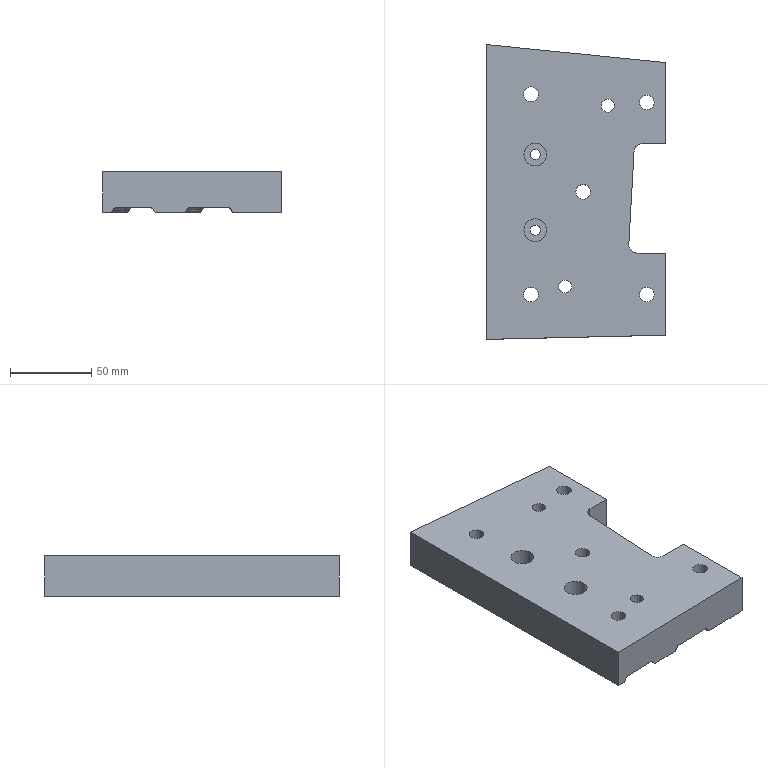Part | NX | features solid 2 | 1 solid | 122 faces | box 110 x 181.223 x 25.004 mm | volume 386395 mm3 | cylinder 58 | plane 27 | torus 23 | spline 14 | commonest cylinder face diameters 4 x21 5 x12 9 x5 14.5 x5 3 x3 6 x3